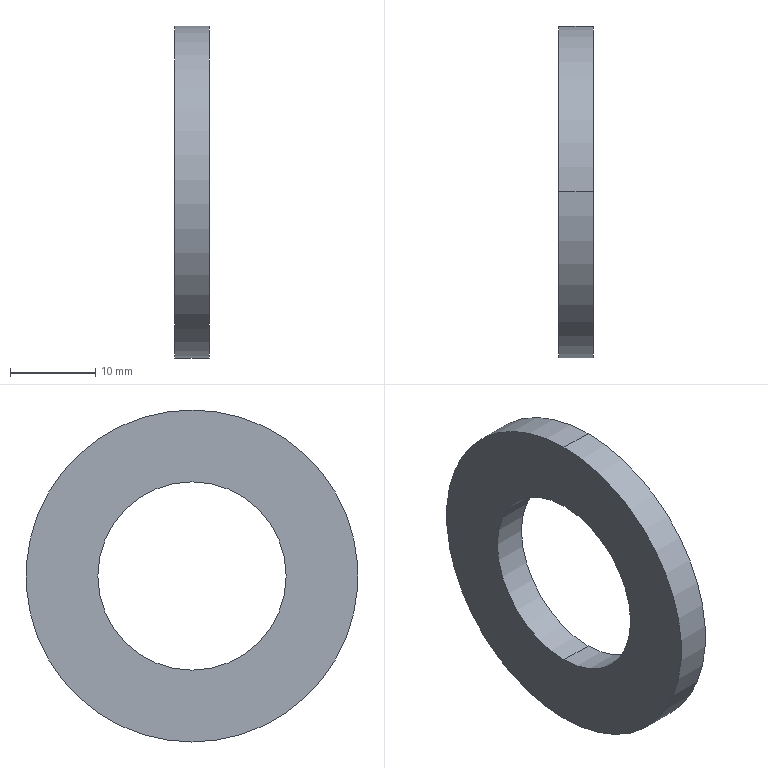Part | STEP file | flat washer narrow_am_B18.22M - Plain washer, 20 mm, narrow | 1 solid | 6 faces | box 4 x 39 x 39 mm | volume 3240 mm3 | cylinder 4 | plane 2 | commonest cylinder face diameters 22.13 x2 39 x2
STEP:
#1=CARTESIAN_POINT('',(0.,0.,0.));
#2=DIRECTION('',(0.,0.,1.));
#3=DIRECTION('',(1.,0.,0.));
#4=AXIS2_PLACEMENT_3D('',#1,#2,#3);
#5=CARTESIAN_POINT('',(0.,0.,19.5));
#6=VERTEX_POINT('',#5);
#7=CARTESIAN_POINT('',(0.,0.,-19.5));
#8=VERTEX_POINT('',#7);
#9=CARTESIAN_POINT('',(0.,0.,0.));
#10=DIRECTION('',(-1.,0.,0.));
#11=DIRECTION('',(0.,0.,1.));
#12=AXIS2_PLACEMENT_3D('',#9,#10,#11);
#13=CIRCLE('',#12,19.5);
#14=CARTESIAN_POINT('',(-34.925,0.,0.));
#15=DIRECTION('',(-1.,0.,0.));
#16=DIRECTION('',(0.,0.,1.));
#17=AXIS2_PLACEMENT_3D('',#14,#15,#16);
#18=CYLINDRICAL_SURFACE('',#17,19.5);
#19=CARTESIAN_POINT('',(0.,-34.925));
#20=DIRECTION('',(1.,0.));
#21=VECTOR('',#20,1.);
#22=LINE('',#19,#21);
#23=(GEOMETRIC_REPRESENTATION_CONTEXT(2)PARAMETRIC_REPRESENTATION_CONTEXT()REPRESENTATION_CONTEXT('',''));
#24=DEFINITIONAL_REPRESENTATION('',(#22),#23);
#25=PCURVE('',#18,#24);
#26=CARTESIAN_POINT('',(0.,11.065,0.));
#27=DIRECTION('',(-1.,0.,0.));
#28=DIRECTION('',(0.,0.,1.));
#29=AXIS2_PLACEMENT_3D('',#26,#27,#28);
#30=PLANE('',#29);
#31=CARTESIAN_POINT('',(0.,-11.065));
#32=DIRECTION('',(1.,0.));
#33=AXIS2_PLACEMENT_2D('',#31,#32);
#34=CIRCLE('',#33,19.5);
#35=(GEOMETRIC_REPRESENTATION_CONTEXT(2)PARAMETRIC_REPRESENTATION_CONTEXT()REPRESENTATION_CONTEXT('',''));
#36=DEFINITIONAL_REPRESENTATION('',(#34),#35);
#37=PCURVE('',#30,#36);
#38=SURFACE_CURVE('',#13,(#25,#37),.PCURVE_S1.);
#39=EDGE_CURVE('',#6,#8,#38,.T.);
#40=ORIENTED_EDGE('',*,*,#39,.T.);
#41=CARTESIAN_POINT('',(-4.,0.,-19.5));
#42=VERTEX_POINT('',#41);
#43=CARTESIAN_POINT('',(-34.925,0.,-19.5));
#44=DIRECTION('',(-1.,0.,0.));
#45=VECTOR('',#44,1.);
#46=LINE('',#43,#45);
#47=CARTESIAN_POINT('',(3.142,0.));
#48=DIRECTION('',(0.,1.));
#49=VECTOR('',#48,1.);
#50=LINE('',#47,#49);
#51=(GEOMETRIC_REPRESENTATION_CONTEXT(2)PARAMETRIC_REPRESENTATION_CONTEXT()REPRESENTATION_CONTEXT('',''));
#52=DEFINITIONAL_REPRESENTATION('',(#50),#51);
#53=PCURVE('',#18,#52);
#54=CARTESIAN_POINT('',(-34.925,0.,0.));
#55=DIRECTION('',(-1.,0.,0.));
#56=DIRECTION('',(0.,0.,1.));
#57=AXIS2_PLACEMENT_3D('',#54,#55,#56);
#58=CYLINDRICAL_SURFACE('',#57,19.5);
#59=CARTESIAN_POINT('',(3.142,0.));
#60=DIRECTION('',(0.,1.));
#61=VECTOR('',#60,1.);
#62=LINE('',#59,#61);
#63=(GEOMETRIC_REPRESENTATION_CONTEXT(2)PARAMETRIC_REPRESENTATION_CONTEXT()REPRESENTATION_CONTEXT('',''));
#64=DEFINITIONAL_REPRESENTATION('',(#62),#63);
#65=PCURVE('',#58,#64);
#66=SURFACE_CURVE('',#46,(#53,#65),.PCURVE_S1.);
#67=EDGE_CURVE('',#8,#42,#66,.T.);
#68=ORIENTED_EDGE('',*,*,#67,.T.);
#69=CARTESIAN_POINT('',(-4.,0.,19.5));
#70=VERTEX_POINT('',#69);
#71=CARTESIAN_POINT('',(-4.,0.,0.));
#72=DIRECTION('',(-1.,0.,0.));
#73=DIRECTION('',(0.,0.,1.));
#74=AXIS2_PLACEMENT_3D('',#71,#72,#73);
#75=CIRCLE('',#74,19.5);
#76=CARTESIAN_POINT('',(0.,-30.925));
#77=DIRECTION('',(1.,0.));
#78=VECTOR('',#77,1.);
#79=LINE('',#76,#78);
#80=(GEOMETRIC_REPRESENTATION_CONTEXT(2)PARAMETRIC_REPRESENTATION_CONTEXT()REPRESENTATION_CONTEXT('',''));
#81=DEFINITIONAL_REPRESENTATION('',(#79),#80);
#82=PCURVE('',#18,#81);
#83=CARTESIAN_POINT('',(-4.,19.5,0.));
#84=DIRECTION('',(1.,0.,0.));
#85=DIRECTION('',(0.,0.,-1.));
#86=AXIS2_PLACEMENT_3D('',#83,#84,#85);
#87=PLANE('',#86);
#88=CARTESIAN_POINT('',(-19.5,-19.5));
#89=CARTESIAN_POINT('',(-19.5,14.275));
#90=CARTESIAN_POINT('',(9.75,-2.613));
#91=CARTESIAN_POINT('',(39.,-19.5));
#92=CARTESIAN_POINT('',(9.75,-36.387));
#93=CARTESIAN_POINT('',(-19.5,-53.275));
#94=CARTESIAN_POINT('',(-19.5,-19.5));
#95=(BOUNDED_CURVE()B_SPLINE_CURVE(2,(#88,#89,#90,#91,#92,#93,#94),.UNSPECIFIED.,.T.,.F.)B_SPLINE_CURVE_WITH_KNOTS((1,2,2,2,2,1),(-2.094,0.,2.094,4.189,6.283,8.378),.UNSPECIFIED.)CURVE()GEOMETRIC_REPRESENTATION_ITEM()RATIONAL_B_SPLINE_CURVE((1.,0.5,1.,0.5,1.,0.5,1.))REPRESENTATION_ITEM(''));
#96=(GEOMETRIC_REPRESENTATION_CONTEXT(2)PARAMETRIC_REPRESENTATION_CONTEXT()REPRESENTATION_CONTEXT('',''));
#97=DEFINITIONAL_REPRESENTATION('',(#95),#96);
#98=PCURVE('',#87,#97);
#99=SURFACE_CURVE('',#75,(#82,#98),.PCURVE_S1.);
#100=EDGE_CURVE('',#70,#42,#99,.T.);
#101=ORIENTED_EDGE('',*,*,#100,.F.);
#102=CARTESIAN_POINT('',(-34.925,0.,19.5));
#103=DIRECTION('',(-1.,0.,0.));
#104=VECTOR('',#103,1.);
#105=LINE('',#102,#104);
#106=CARTESIAN_POINT('',(0.,0.));
#107=DIRECTION('',(0.,1.));
#108=VECTOR('',#107,1.);
#109=LINE('',#106,#108);
#110=(GEOMETRIC_REPRESENTATION_CONTEXT(2)PARAMETRIC_REPRESENTATION_CONTEXT()REPRESENTATION_CONTEXT('',''));
#111=DEFINITIONAL_REPRESENTATION('',(#109),#110);
#112=PCURVE('',#18,#111);
#113=CARTESIAN_POINT('',(6.283,0.));
#114=DIRECTION('',(0.,1.));
#115=VECTOR('',#114,1.);
#116=LINE('',#113,#115);
#117=(GEOMETRIC_REPRESENTATION_CONTEXT(2)PARAMETRIC_REPRESENTATION_CONTEXT()REPRESENTATION_CONTEXT('',''));
#118=DEFINITIONAL_REPRESENTATION('',(#116),#117);
#119=PCURVE('',#58,#118);
#120=SURFACE_CURVE('',#105,(#112,#119),.PCURVE_S1.);
#121=EDGE_CURVE('',#6,#70,#120,.T.);
#122=ORIENTED_EDGE('',*,*,#121,.F.);
#123=EDGE_LOOP('',(#40,#68,#101,#122));
#124=FACE_BOUND('',#123,.T.);
#125=ADVANCED_FACE('',(#124),#18,.T.);
#126=CARTESIAN_POINT('',(0.,0.,11.065));
#127=VERTEX_POINT('',#126);
#128=CARTESIAN_POINT('',(-4.,0.,11.065));
#129=VERTEX_POINT('',#128);
#130=CARTESIAN_POINT('',(-34.925,0.,11.065));
#131=DIRECTION('',(-1.,0.,0.));
#132=VECTOR('',#131,1.);
#133=LINE('',#130,#132);
#134=CARTESIAN_POINT('',(-34.925,0.,0.));
#135=DIRECTION('',(-1.,0.,0.));
#136=DIRECTION('',(0.,0.,1.));
#137=AXIS2_PLACEMENT_3D('',#134,#135,#136);
#138=CYLINDRICAL_SURFACE('',#137,11.065);
#139=CARTESIAN_POINT('',(6.283,0.));
#140=DIRECTION('',(0.,1.));
#141=VECTOR('',#140,1.);
#142=LINE('',#139,#141);
#143=(GEOMETRIC_REPRESENTATION_CONTEXT(2)PARAMETRIC_REPRESENTATION_CONTEXT()REPRESENTATION_CONTEXT('',''));
#144=DEFINITIONAL_REPRESENTATION('',(#142),#143);
#145=PCURVE('',#138,#144);
#146=CARTESIAN_POINT('',(-34.925,0.,0.));
#147=DIRECTION('',(-1.,0.,0.));
#148=DIRECTION('',(0.,0.,1.));
#149=AXIS2_PLACEMENT_3D('',#146,#147,#148);
#150=CYLINDRICAL_SURFACE('',#149,11.065);
#151=CARTESIAN_POINT('',(0.,0.));
#152=DIRECTION('',(0.,1.));
#153=VECTOR('',#152,1.);
#154=LINE('',#151,#153);
#155=(GEOMETRIC_REPRESENTATION_CONTEXT(2)PARAMETRIC_REPRESENTATION_CONTEXT()REPRESENTATION_CONTEXT('',''));
#156=DEFINITIONAL_REPRESENTATION('',(#154),#155);
#157=PCURVE('',#150,#156);
#158=SURFACE_CURVE('',#133,(#145,#157),.PCURVE_S1.);
#159=EDGE_CURVE('',#127,#129,#158,.T.);
#160=ORIENTED_EDGE('',*,*,#159,.T.);
#161=CARTESIAN_POINT('',(-4.,0.,-11.065));
#162=VERTEX_POINT('',#161);
#163=CARTESIAN_POINT('',(-4.,0.,0.));
#164=DIRECTION('',(-1.,0.,0.));
#165=DIRECTION('',(0.,0.,1.));
#166=AXIS2_PLACEMENT_3D('',#163,#164,#165);
#167=CIRCLE('',#166,11.065);
#168=CARTESIAN_POINT('',(0.,-30.925));
#169=DIRECTION('',(1.,0.));
#170=VECTOR('',#169,1.);
#171=LINE('',#168,#170);
#172=(GEOMETRIC_REPRESENTATION_CONTEXT(2)PARAMETRIC_REPRESENTATION_CONTEXT()REPRESENTATION_CONTEXT('',''));
#173=DEFINITIONAL_REPRESENTATION('',(#171),#172);
#174=PCURVE('',#138,#173);
#175=CARTESIAN_POINT('',(-11.065,-19.5));
#176=CARTESIAN_POINT('',(-11.065,-0.3349));
#177=CARTESIAN_POINT('',(5.532,-9.917));
#178=CARTESIAN_POINT('',(22.13,-19.5));
#179=CARTESIAN_POINT('',(5.532,-29.083));
#180=CARTESIAN_POINT('',(-11.065,-38.665));
#181=CARTESIAN_POINT('',(-11.065,-19.5));
#182=(BOUNDED_CURVE()B_SPLINE_CURVE(2,(#175,#176,#177,#178,#179,#180,#181),.UNSPECIFIED.,.T.,.F.)B_SPLINE_CURVE_WITH_KNOTS((1,2,2,2,2,1),(-2.094,0.,2.094,4.189,6.283,8.378),.UNSPECIFIED.)CURVE()GEOMETRIC_REPRESENTATION_ITEM()RATIONAL_B_SPLINE_CURVE((1.,0.5,1.,0.5,1.,0.5,1.))REPRESENTATION_ITEM(''));
#183=(GEOMETRIC_REPRESENTATION_CONTEXT(2)PARAMETRIC_REPRESENTATION_CONTEXT()REPRESENTATION_CONTEXT('',''));
#184=DEFINITIONAL_REPRESENTATION('',(#182),#183);
#185=PCURVE('',#87,#184);
#186=SURFACE_CURVE('',#167,(#174,#185),.PCURVE_S1.);
#187=EDGE_CURVE('',#162,#129,#186,.T.);
#188=ORIENTED_EDGE('',*,*,#187,.F.);
#189=CARTESIAN_POINT('',(0.,0.,-11.065));
#190=VERTEX_POINT('',#189);
#191=CARTESIAN_POINT('',(-34.925,0.,-11.065));
#192=DIRECTION('',(-1.,0.,0.));
#193=VECTOR('',#192,1.);
#194=LINE('',#191,#193);
#195=CARTESIAN_POINT('',(3.142,0.));
#196=DIRECTION('',(0.,1.));
#197=VECTOR('',#196,1.);
#198=LINE('',#195,#197);
#199=(GEOMETRIC_REPRESENTATION_CONTEXT(2)PARAMETRIC_REPRESENTATION_CONTEXT()REPRESENTATION_CONTEXT('',''));
#200=DEFINITIONAL_REPRESENTATION('',(#198),#199);
#201=PCURVE('',#138,#200);
#202=CARTESIAN_POINT('',(3.142,0.));
#203=DIRECTION('',(0.,1.));
#204=VECTOR('',#203,1.);
#205=LINE('',#202,#204);
#206=(GEOMETRIC_REPRESENTATION_CONTEXT(2)PARAMETRIC_REPRESENTATION_CONTEXT()REPRESENTATION_CONTEXT('',''));
#207=DEFINITIONAL_REPRESENTATION('',(#205),#206);
#208=PCURVE('',#150,#207);
#209=SURFACE_CURVE('',#194,(#201,#208),.PCURVE_S1.);
#210=EDGE_CURVE('',#190,#162,#209,.T.);
#211=ORIENTED_EDGE('',*,*,#210,.F.);
#212=CARTESIAN_POINT('',(0.,0.,0.));
#213=DIRECTION('',(-1.,0.,0.));
#214=DIRECTION('',(0.,0.,1.));
#215=AXIS2_PLACEMENT_3D('',#212,#213,#214);
#216=CIRCLE('',#215,11.065);
#217=CARTESIAN_POINT('',(0.,-34.925));
#218=DIRECTION('',(1.,0.));
#219=VECTOR('',#218,1.);
#220=LINE('',#217,#219);
#221=(GEOMETRIC_REPRESENTATION_CONTEXT(2)PARAMETRIC_REPRESENTATION_CONTEXT()REPRESENTATION_CONTEXT('',''));
#222=DEFINITIONAL_REPRESENTATION('',(#220),#221);
#223=PCURVE('',#138,#222);
#224=CARTESIAN_POINT('',(0.,-11.065));
#225=DIRECTION('',(1.,0.));
#226=AXIS2_PLACEMENT_2D('',#224,#225);
#227=CIRCLE('',#226,11.065);
#228=(GEOMETRIC_REPRESENTATION_CONTEXT(2)PARAMETRIC_REPRESENTATION_CONTEXT()REPRESENTATION_CONTEXT('',''));
#229=DEFINITIONAL_REPRESENTATION('',(#227),#228);
#230=PCURVE('',#30,#229);
#231=SURFACE_CURVE('',#216,(#223,#230),.PCURVE_S1.);
#232=EDGE_CURVE('',#190,#127,#231,.T.);
#233=ORIENTED_EDGE('',*,*,#232,.T.);
#234=EDGE_LOOP('',(#160,#188,#211,#233));
#235=FACE_BOUND('',#234,.F.);
#236=ADVANCED_FACE('',(#235),#138,.F.);
#237=CARTESIAN_POINT('',(-4.,0.,0.));
#238=DIRECTION('',(-1.,0.,0.));
#239=DIRECTION('',(0.,0.,1.));
#240=AXIS2_PLACEMENT_3D('',#237,#238,#239);
#241=CIRCLE('',#240,11.065);
#242=CARTESIAN_POINT('',(0.,-30.925));
#243=DIRECTION('',(1.,0.));
#244=VECTOR('',#243,1.);
#245=LINE('',#242,#244);
#246=(GEOMETRIC_REPRESENTATION_CONTEXT(2)PARAMETRIC_REPRESENTATION_CONTEXT()REPRESENTATION_CONTEXT('',''));
#247=DEFINITIONAL_REPRESENTATION('',(#245),#246);
#248=PCURVE('',#150,#247);
#249=CARTESIAN_POINT('',(-11.065,-19.5));
#250=CARTESIAN_POINT('',(-11.065,-0.3349));
#251=CARTESIAN_POINT('',(5.532,-9.917));
#252=CARTESIAN_POINT('',(22.13,-19.5));
#253=CARTESIAN_POINT('',(5.532,-29.083));
#254=CARTESIAN_POINT('',(-11.065,-38.665));
#255=CARTESIAN_POINT('',(-11.065,-19.5));
#256=(BOUNDED_CURVE()B_SPLINE_CURVE(2,(#249,#250,#251,#252,#253,#254,#255),.UNSPECIFIED.,.T.,.F.)B_SPLINE_CURVE_WITH_KNOTS((1,2,2,2,2,1),(-2.094,0.,2.094,4.189,6.283,8.378),.UNSPECIFIED.)CURVE()GEOMETRIC_REPRESENTATION_ITEM()RATIONAL_B_SPLINE_CURVE((1.,0.5,1.,0.5,1.,0.5,1.))REPRESENTATION_ITEM(''));
#257=(GEOMETRIC_REPRESENTATION_CONTEXT(2)PARAMETRIC_REPRESENTATION_CONTEXT()REPRESENTATION_CONTEXT('',''));
#258=DEFINITIONAL_REPRESENTATION('',(#256),#257);
#259=PCURVE('',#87,#258);
#260=SURFACE_CURVE('',#241,(#248,#259),.PCURVE_S1.);
#261=EDGE_CURVE('',#129,#162,#260,.T.);
#262=ORIENTED_EDGE('',*,*,#261,.F.);
#263=ORIENTED_EDGE('',*,*,#159,.F.);
#264=CARTESIAN_POINT('',(0.,0.,0.));
#265=DIRECTION('',(-1.,0.,0.));
#266=DIRECTION('',(0.,0.,1.));
#267=AXIS2_PLACEMENT_3D('',#264,#265,#266);
#268=CIRCLE('',#267,11.065);
#269=CARTESIAN_POINT('',(0.,-34.925));
#270=DIRECTION('',(1.,0.));
#271=VECTOR('',#270,1.);
#272=LINE('',#269,#271);
#273=(GEOMETRIC_REPRESENTATION_CONTEXT(2)PARAMETRIC_REPRESENTATION_CONTEXT()REPRESENTATION_CONTEXT('',''));
#274=DEFINITIONAL_REPRESENTATION('',(#272),#273);
#275=PCURVE('',#150,#274);
#276=CARTESIAN_POINT('',(0.,-11.065));
#277=DIRECTION('',(1.,0.));
#278=AXIS2_PLACEMENT_2D('',#276,#277);
#279=CIRCLE('',#278,11.065);
#280=(GEOMETRIC_REPRESENTATION_CONTEXT(2)PARAMETRIC_REPRESENTATION_CONTEXT()REPRESENTATION_CONTEXT('',''));
#281=DEFINITIONAL_REPRESENTATION('',(#279),#280);
#282=PCURVE('',#30,#281);
#283=SURFACE_CURVE('',#268,(#275,#282),.PCURVE_S1.);
#284=EDGE_CURVE('',#127,#190,#283,.T.);
#285=ORIENTED_EDGE('',*,*,#284,.T.);
#286=ORIENTED_EDGE('',*,*,#210,.T.);
#287=EDGE_LOOP('',(#262,#263,#285,#286));
#288=FACE_BOUND('',#287,.F.);
#289=ADVANCED_FACE('',(#288),#150,.F.);
#290=ORIENTED_EDGE('',*,*,#39,.F.);
#291=CARTESIAN_POINT('',(0.,0.,0.));
#292=DIRECTION('',(-1.,0.,0.));
#293=DIRECTION('',(0.,0.,1.));
#294=AXIS2_PLACEMENT_3D('',#291,#292,#293);
#295=CIRCLE('',#294,19.5);
#296=CARTESIAN_POINT('',(0.,-11.065));
#297=DIRECTION('',(1.,0.));
#298=AXIS2_PLACEMENT_2D('',#296,#297);
#299=CIRCLE('',#298,19.5);
#300=(GEOMETRIC_REPRESENTATION_CONTEXT(2)PARAMETRIC_REPRESENTATION_CONTEXT()REPRESENTATION_CONTEXT('',''));
#301=DEFINITIONAL_REPRESENTATION('',(#299),#300);
#302=PCURVE('',#30,#301);
#303=CARTESIAN_POINT('',(0.,-34.925));
#304=DIRECTION('',(1.,0.));
#305=VECTOR('',#304,1.);
#306=LINE('',#303,#305);
#307=(GEOMETRIC_REPRESENTATION_CONTEXT(2)PARAMETRIC_REPRESENTATION_CONTEXT()REPRESENTATION_CONTEXT('',''));
#308=DEFINITIONAL_REPRESENTATION('',(#306),#307);
#309=PCURVE('',#58,#308);
#310=SURFACE_CURVE('',#295,(#302,#309),.PCURVE_S1.);
#311=EDGE_CURVE('',#8,#6,#310,.T.);
#312=ORIENTED_EDGE('',*,*,#311,.F.);
#313=EDGE_LOOP('',(#290,#312));
#314=FACE_BOUND('',#313,.T.);
#315=ORIENTED_EDGE('',*,*,#284,.T.);
#316=ORIENTED_EDGE('',*,*,#232,.T.);
#317=EDGE_LOOP('',(#315,#316));
#318=FACE_BOUND('',#317,.T.);
#319=ADVANCED_FACE('',(#314,#318),#30,.F.);
#320=ORIENTED_EDGE('',*,*,#67,.F.);
#321=ORIENTED_EDGE('',*,*,#311,.T.);
#322=ORIENTED_EDGE('',*,*,#121,.T.);
#323=CARTESIAN_POINT('',(-4.,0.,0.));
#324=DIRECTION('',(-1.,0.,0.));
#325=DIRECTION('',(0.,0.,1.));
#326=AXIS2_PLACEMENT_3D('',#323,#324,#325);
#327=CIRCLE('',#326,19.5);
#328=CARTESIAN_POINT('',(0.,-30.925));
#329=DIRECTION('',(1.,0.));
#330=VECTOR('',#329,1.);
#331=LINE('',#328,#330);
#332=(GEOMETRIC_REPRESENTATION_CONTEXT(2)PARAMETRIC_REPRESENTATION_CONTEXT()REPRESENTATION_CONTEXT('',''));
#333=DEFINITIONAL_REPRESENTATION('',(#331),#332);
#334=PCURVE('',#58,#333);
#335=CARTESIAN_POINT('',(-19.5,-19.5));
#336=CARTESIAN_POINT('',(-19.5,14.275));
#337=CARTESIAN_POINT('',(9.75,-2.613));
#338=CARTESIAN_POINT('',(39.,-19.5));
#339=CARTESIAN_POINT('',(9.75,-36.387));
#340=CARTESIAN_POINT('',(-19.5,-53.275));
#341=CARTESIAN_POINT('',(-19.5,-19.5));
#342=(BOUNDED_CURVE()B_SPLINE_CURVE(2,(#335,#336,#337,#338,#339,#340,#341),.UNSPECIFIED.,.T.,.F.)B_SPLINE_CURVE_WITH_KNOTS((1,2,2,2,2,1),(-2.094,0.,2.094,4.189,6.283,8.378),.UNSPECIFIED.)CURVE()GEOMETRIC_REPRESENTATION_ITEM()RATIONAL_B_SPLINE_CURVE((1.,0.5,1.,0.5,1.,0.5,1.))REPRESENTATION_ITEM(''));
#343=(GEOMETRIC_REPRESENTATION_CONTEXT(2)PARAMETRIC_REPRESENTATION_CONTEXT()REPRESENTATION_CONTEXT('',''));
#344=DEFINITIONAL_REPRESENTATION('',(#342),#343);
#345=PCURVE('',#87,#344);
#346=SURFACE_CURVE('',#327,(#334,#345),.PCURVE_S1.);
#347=EDGE_CURVE('',#42,#70,#346,.T.);
#348=ORIENTED_EDGE('',*,*,#347,.F.);
#349=EDGE_LOOP('',(#320,#321,#322,#348));
#350=FACE_BOUND('',#349,.T.);
#351=ADVANCED_FACE('',(#350),#58,.T.);
#352=ORIENTED_EDGE('',*,*,#261,.F.);
#353=ORIENTED_EDGE('',*,*,#187,.F.);
#354=EDGE_LOOP('',(#352,#353));
#355=FACE_BOUND('',#354,.T.);
#356=ORIENTED_EDGE('',*,*,#100,.T.);
#357=ORIENTED_EDGE('',*,*,#347,.T.);
#358=EDGE_LOOP('',(#356,#357));
#359=FACE_BOUND('',#358,.T.);
#360=ADVANCED_FACE('',(#355,#359),#87,.F.);
#361=CLOSED_SHELL('',(#125,#236,#289,#319,#351,#360));
#362=MANIFOLD_SOLID_BREP('',#361);
#363=(LENGTH_UNIT()NAMED_UNIT(*)SI_UNIT(.MILLI.,.METRE.));
#364=UNCERTAINTY_MEASURE_WITH_UNIT(LENGTH_MEASURE(0.0000001),#363,'','');
#365=(NAMED_UNIT(*)PLANE_ANGLE_UNIT()SI_UNIT($,.RADIAN.));
#366=(NAMED_UNIT(*)SI_UNIT($,.STERADIAN.)SOLID_ANGLE_UNIT());
#367=(GEOMETRIC_REPRESENTATION_CONTEXT(3)GLOBAL_UNCERTAINTY_ASSIGNED_CONTEXT((#364))GLOBAL_UNIT_ASSIGNED_CONTEXT((#363,#365,#366))REPRESENTATION_CONTEXT('',''));
#368=ADVANCED_BREP_SHAPE_REPRESENTATION('',(#4,#362),#367);